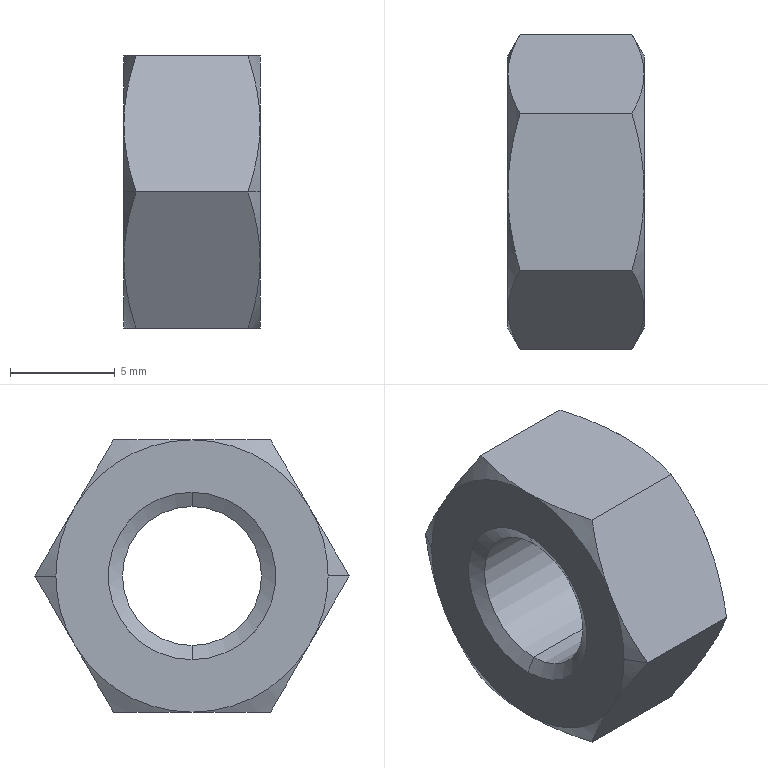Part | STEP file | KS B 1012 - M 8 | 1 solid | 30 faces | box 6.5 x 15.011 x 13 mm | volume 715.11 mm3 | cone 20 | plane 8 | cylinder 2 | commonest cylinder face diameters 6.647 x2